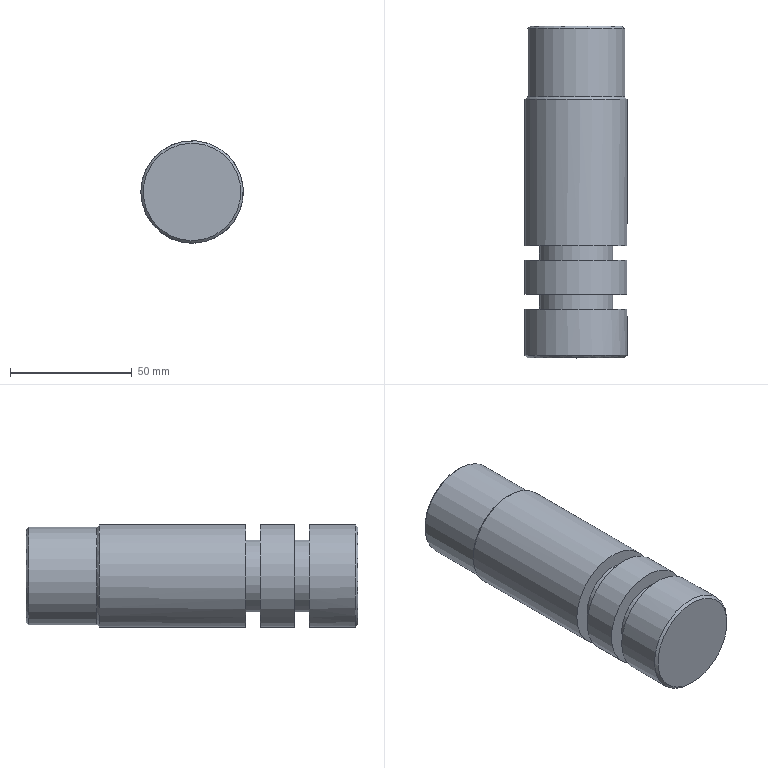Part | NX | features solid 2 | 1 solid | 15 faces | box 42 x 136 x 42 mm | volume 176350 mm3 | plane 6 | cylinder 6 | cone 3 | commonest cylinder face diameters 42 x3 30 x2 40 x1
STEP:
#1=CARTESIAN_POINT('',(-801.,-555.,180.));
#2=VERTEX_POINT('',#1);
#3=CARTESIAN_POINT('',(-780.,-555.,180.));
#4=DIRECTION('',(0.,1.,0.));
#5=DIRECTION('',(-1.,0.,0.));
#6=AXIS2_PLACEMENT_3D('',#3,#4,#5);
#7=CIRCLE('',#6,21.);
#8=EDGE_CURVE('',#2,#2,#7,.T.);
#9=ORIENTED_EDGE('',*,*,#8,.F.);
#10=EDGE_LOOP('',(#9));
#11=FACE_BOUND('',#10,.T.);
#12=CARTESIAN_POINT('',(-795.,-555.,180.));
#13=VERTEX_POINT('',#12);
#14=CARTESIAN_POINT('',(-780.,-555.,180.));
#15=DIRECTION('',(0.,1.,0.));
#16=DIRECTION('',(-1.,0.,0.));
#17=AXIS2_PLACEMENT_3D('',#14,#15,#16);
#18=CIRCLE('',#17,15.);
#19=EDGE_CURVE('',#13,#13,#18,.T.);
#20=ORIENTED_EDGE('',*,*,#19,.T.);
#21=EDGE_LOOP('',(#20));
#22=FACE_BOUND('',#21,.T.);
#23=CARTESIAN_POINT('',(-780.,-555.,180.));
#24=DIRECTION('',(0.,-1.,0.));
#25=DIRECTION('',(0.,0.,-1.));
#26=AXIS2_PLACEMENT_3D('',#23,#24,#25);
#27=PLANE('',#26);
#28=ADVANCED_FACE('',(#11,#22),#27,.T.);
#29=CARTESIAN_POINT('',(-801.,-535.,180.));
#30=VERTEX_POINT('',#29);
#31=CARTESIAN_POINT('',(-780.,-535.,180.));
#32=DIRECTION('',(0.,1.,0.));
#33=DIRECTION('',(-1.,0.,0.));
#34=AXIS2_PLACEMENT_3D('',#31,#32,#33);
#35=CIRCLE('',#34,21.);
#36=EDGE_CURVE('',#30,#30,#35,.T.);
#37=ORIENTED_EDGE('',*,*,#36,.F.);
#38=EDGE_LOOP('',(#37));
#39=FACE_BOUND('',#38,.T.);
#40=CARTESIAN_POINT('',(-795.,-535.,180.));
#41=VERTEX_POINT('',#40);
#42=CARTESIAN_POINT('',(-780.,-535.,180.));
#43=DIRECTION('',(0.,1.,0.));
#44=DIRECTION('',(-1.,0.,0.));
#45=AXIS2_PLACEMENT_3D('',#42,#43,#44);
#46=CIRCLE('',#45,15.);
#47=EDGE_CURVE('',#41,#41,#46,.T.);
#48=ORIENTED_EDGE('',*,*,#47,.T.);
#49=EDGE_LOOP('',(#48));
#50=FACE_BOUND('',#49,.T.);
#51=CARTESIAN_POINT('',(-780.,-535.,180.));
#52=DIRECTION('',(0.,-1.,0.));
#53=DIRECTION('',(0.,0.,-1.));
#54=AXIS2_PLACEMENT_3D('',#51,#52,#53);
#55=PLANE('',#54);
#56=ADVANCED_FACE('',(#39,#50),#55,.T.);
#57=CARTESIAN_POINT('',(-801.,-475.,180.));
#58=VERTEX_POINT('',#57);
#59=CARTESIAN_POINT('',(-780.,-475.,180.));
#60=DIRECTION('',(0.,1.,0.));
#61=DIRECTION('',(-1.,0.,0.));
#62=AXIS2_PLACEMENT_3D('',#59,#60,#61);
#63=CIRCLE('',#62,21.);
#64=EDGE_CURVE('',#58,#58,#63,.T.);
#65=ORIENTED_EDGE('',*,*,#64,.F.);
#66=EDGE_LOOP('',(#65));
#67=FACE_BOUND('',#66,.T.);
#68=ORIENTED_EDGE('',*,*,#36,.T.);
#69=EDGE_LOOP('',(#68));
#70=FACE_BOUND('',#69,.T.);
#71=CARTESIAN_POINT('',(-780.,-535.,180.));
#72=DIRECTION('',(0.,1.,0.));
#73=DIRECTION('',(0.,0.,1.));
#74=AXIS2_PLACEMENT_3D('',#71,#72,#73);
#75=CYLINDRICAL_SURFACE('',#74,21.);
#76=ADVANCED_FACE('',(#67,#70),#75,.T.);
#77=CARTESIAN_POINT('',(-795.,-541.,180.));
#78=VERTEX_POINT('',#77);
#79=CARTESIAN_POINT('',(-780.,-541.,180.));
#80=DIRECTION('',(0.,1.,0.));
#81=DIRECTION('',(-1.,0.,0.));
#82=AXIS2_PLACEMENT_3D('',#79,#80,#81);
#83=CIRCLE('',#82,15.);
#84=EDGE_CURVE('',#78,#78,#83,.T.);
#85=ORIENTED_EDGE('',*,*,#84,.T.);
#86=EDGE_LOOP('',(#85));
#87=FACE_BOUND('',#86,.T.);
#88=ORIENTED_EDGE('',*,*,#47,.F.);
#89=EDGE_LOOP('',(#88));
#90=FACE_BOUND('',#89,.T.);
#91=CARTESIAN_POINT('',(-780.,-541.,180.));
#92=DIRECTION('',(0.,1.,0.));
#93=DIRECTION('',(0.,0.,1.));
#94=AXIS2_PLACEMENT_3D('',#91,#92,#93);
#95=CYLINDRICAL_SURFACE('',#94,15.);
#96=ADVANCED_FACE('',(#87,#90),#95,.T.);
#97=CARTESIAN_POINT('',(-801.,-541.,180.));
#98=VERTEX_POINT('',#97);
#99=CARTESIAN_POINT('',(-780.,-541.,180.));
#100=DIRECTION('',(0.,1.,0.));
#101=DIRECTION('',(-1.,0.,0.));
#102=AXIS2_PLACEMENT_3D('',#99,#100,#101);
#103=CIRCLE('',#102,21.);
#104=EDGE_CURVE('',#98,#98,#103,.T.);
#105=ORIENTED_EDGE('',*,*,#104,.T.);
#106=EDGE_LOOP('',(#105));
#107=FACE_BOUND('',#106,.T.);
#108=ORIENTED_EDGE('',*,*,#84,.F.);
#109=EDGE_LOOP('',(#108));
#110=FACE_BOUND('',#109,.T.);
#111=CARTESIAN_POINT('',(-780.,-541.,180.));
#112=DIRECTION('',(0.,-1.,0.));
#113=DIRECTION('',(0.,0.,-1.));
#114=AXIS2_PLACEMENT_3D('',#111,#112,#113);
#115=PLANE('',#114);
#116=ADVANCED_FACE('',(#107,#110),#115,.F.);
#117=ORIENTED_EDGE('',*,*,#8,.T.);
#118=EDGE_LOOP('',(#117));
#119=FACE_BOUND('',#118,.T.);
#120=ORIENTED_EDGE('',*,*,#104,.F.);
#121=EDGE_LOOP('',(#120));
#122=FACE_BOUND('',#121,.T.);
#123=CARTESIAN_POINT('',(-780.,-555.,180.));
#124=DIRECTION('',(0.,1.,0.));
#125=DIRECTION('',(0.,0.,1.));
#126=AXIS2_PLACEMENT_3D('',#123,#124,#125);
#127=CYLINDRICAL_SURFACE('',#126,21.);
#128=ADVANCED_FACE('',(#119,#122),#127,.T.);
#129=CARTESIAN_POINT('',(-795.,-561.,180.));
#130=VERTEX_POINT('',#129);
#131=CARTESIAN_POINT('',(-780.,-561.,180.));
#132=DIRECTION('',(0.,1.,0.));
#133=DIRECTION('',(-1.,0.,0.));
#134=AXIS2_PLACEMENT_3D('',#131,#132,#133);
#135=CIRCLE('',#134,15.);
#136=EDGE_CURVE('',#130,#130,#135,.T.);
#137=ORIENTED_EDGE('',*,*,#136,.T.);
#138=EDGE_LOOP('',(#137));
#139=FACE_BOUND('',#138,.T.);
#140=ORIENTED_EDGE('',*,*,#19,.F.);
#141=EDGE_LOOP('',(#140));
#142=FACE_BOUND('',#141,.T.);
#143=CARTESIAN_POINT('',(-780.,-561.,180.));
#144=DIRECTION('',(0.,1.,0.));
#145=DIRECTION('',(0.,0.,1.));
#146=AXIS2_PLACEMENT_3D('',#143,#144,#145);
#147=CYLINDRICAL_SURFACE('',#146,15.);
#148=ADVANCED_FACE('',(#139,#142),#147,.T.);
#149=CARTESIAN_POINT('',(-801.,-561.,180.));
#150=VERTEX_POINT('',#149);
#151=CARTESIAN_POINT('',(-780.,-561.,180.));
#152=DIRECTION('',(0.,1.,0.));
#153=DIRECTION('',(-1.,0.,0.));
#154=AXIS2_PLACEMENT_3D('',#151,#152,#153);
#155=CIRCLE('',#154,21.);
#156=EDGE_CURVE('',#150,#150,#155,.T.);
#157=ORIENTED_EDGE('',*,*,#156,.T.);
#158=EDGE_LOOP('',(#157));
#159=FACE_BOUND('',#158,.T.);
#160=ORIENTED_EDGE('',*,*,#136,.F.);
#161=EDGE_LOOP('',(#160));
#162=FACE_BOUND('',#161,.T.);
#163=CARTESIAN_POINT('',(-780.,-561.,180.));
#164=DIRECTION('',(0.,-1.,0.));
#165=DIRECTION('',(0.,0.,-1.));
#166=AXIS2_PLACEMENT_3D('',#163,#164,#165);
#167=PLANE('',#166);
#168=ADVANCED_FACE('',(#159,#162),#167,.F.);
#169=CARTESIAN_POINT('',(-780.,-580.,159.));
#170=VERTEX_POINT('',#169);
#171=CARTESIAN_POINT('',(-780.,-580.,180.));
#172=DIRECTION('',(0.,1.,0.));
#173=DIRECTION('',(0.,0.,-1.));
#174=AXIS2_PLACEMENT_3D('',#171,#172,#173);
#175=CIRCLE('',#174,21.);
#176=EDGE_CURVE('',#170,#170,#175,.F.);
#177=ORIENTED_EDGE('',*,*,#176,.F.);
#178=EDGE_LOOP('',(#177));
#179=FACE_BOUND('',#178,.T.);
#180=ORIENTED_EDGE('',*,*,#156,.F.);
#181=EDGE_LOOP('',(#180));
#182=FACE_BOUND('',#181,.T.);
#183=CARTESIAN_POINT('',(-780.,-581.,180.));
#184=DIRECTION('',(0.,1.,0.));
#185=DIRECTION('',(0.,0.,1.));
#186=AXIS2_PLACEMENT_3D('',#183,#184,#185);
#187=CYLINDRICAL_SURFACE('',#186,21.);
#188=ADVANCED_FACE('',(#179,#182),#187,.T.);
#189=CARTESIAN_POINT('',(-780.,-581.,160.));
#190=VERTEX_POINT('',#189);
#191=CARTESIAN_POINT('',(-780.,-581.,180.));
#192=DIRECTION('',(0.,1.,0.));
#193=DIRECTION('',(0.,0.,-1.));
#194=AXIS2_PLACEMENT_3D('',#191,#192,#193);
#195=CIRCLE('',#194,20.);
#196=EDGE_CURVE('',#190,#190,#195,.T.);
#197=ORIENTED_EDGE('',*,*,#196,.F.);
#198=EDGE_LOOP('',(#197));
#199=FACE_BOUND('',#198,.T.);
#200=CARTESIAN_POINT('',(-780.,-581.,180.));
#201=DIRECTION('',(0.,-1.,0.));
#202=DIRECTION('',(0.,0.,-1.));
#203=AXIS2_PLACEMENT_3D('',#200,#201,#202);
#204=PLANE('',#203);
#205=ADVANCED_FACE('',(#199),#204,.T.);
#206=CARTESIAN_POINT('',(-780.,-474.,160.));
#207=VERTEX_POINT('',#206);
#208=CARTESIAN_POINT('',(-780.,-474.,180.));
#209=DIRECTION('',(0.,1.,0.));
#210=DIRECTION('',(0.,0.,-1.));
#211=AXIS2_PLACEMENT_3D('',#208,#209,#210);
#212=CIRCLE('',#211,20.);
#213=EDGE_CURVE('',#207,#207,#212,.F.);
#214=ORIENTED_EDGE('',*,*,#213,.F.);
#215=EDGE_LOOP('',(#214));
#216=FACE_BOUND('',#215,.T.);
#217=CARTESIAN_POINT('',(-780.,-446.,160.));
#218=VERTEX_POINT('',#217);
#219=CARTESIAN_POINT('',(-780.,-446.,180.));
#220=DIRECTION('',(0.,1.,0.));
#221=DIRECTION('',(0.,0.,-1.));
#222=AXIS2_PLACEMENT_3D('',#219,#220,#221);
#223=CIRCLE('',#222,20.);
#224=EDGE_CURVE('',#218,#218,#223,.T.);
#225=ORIENTED_EDGE('',*,*,#224,.F.);
#226=EDGE_LOOP('',(#225));
#227=FACE_BOUND('',#226,.T.);
#228=CARTESIAN_POINT('',(-780.,-405.,180.));
#229=DIRECTION('',(0.,-1.,0.));
#230=DIRECTION('',(0.,0.,-1.));
#231=AXIS2_PLACEMENT_3D('',#228,#229,#230);
#232=CYLINDRICAL_SURFACE('',#231,20.);
#233=ADVANCED_FACE('',(#216,#227),#232,.T.);
#234=CARTESIAN_POINT('',(-780.,-445.,161.));
#235=VERTEX_POINT('',#234);
#236=CARTESIAN_POINT('',(-780.,-445.,180.));
#237=DIRECTION('',(0.,1.,0.));
#238=DIRECTION('',(0.,0.,-1.));
#239=AXIS2_PLACEMENT_3D('',#236,#237,#238);
#240=CIRCLE('',#239,19.);
#241=EDGE_CURVE('',#235,#235,#240,.F.);
#242=ORIENTED_EDGE('',*,*,#241,.F.);
#243=EDGE_LOOP('',(#242));
#244=FACE_BOUND('',#243,.T.);
#245=CARTESIAN_POINT('',(-780.,-445.,180.));
#246=DIRECTION('',(0.,-1.,0.));
#247=DIRECTION('',(0.,0.,-1.));
#248=AXIS2_PLACEMENT_3D('',#245,#246,#247);
#249=PLANE('',#248);
#250=ADVANCED_FACE('',(#244),#249,.F.);
#251=ORIENTED_EDGE('',*,*,#241,.T.);
#252=EDGE_LOOP('',(#251));
#253=FACE_BOUND('',#252,.T.);
#254=ORIENTED_EDGE('',*,*,#224,.T.);
#255=EDGE_LOOP('',(#254));
#256=FACE_BOUND('',#255,.T.);
#257=CARTESIAN_POINT('',(-780.,-446.,180.));
#258=DIRECTION('',(0.,-1.,0.));
#259=DIRECTION('',(0.,0.,-1.));
#260=AXIS2_PLACEMENT_3D('',#257,#258,#259);
#261=CONICAL_SURFACE('',#260,20.,0.7854);
#262=ADVANCED_FACE('',(#253,#256),#261,.T.);
#263=ORIENTED_EDGE('',*,*,#213,.T.);
#264=EDGE_LOOP('',(#263));
#265=FACE_BOUND('',#264,.T.);
#266=ORIENTED_EDGE('',*,*,#64,.T.);
#267=EDGE_LOOP('',(#266));
#268=FACE_BOUND('',#267,.T.);
#269=CARTESIAN_POINT('',(-780.,-475.,180.));
#270=DIRECTION('',(0.,-1.,0.));
#271=DIRECTION('',(0.,0.,-1.));
#272=AXIS2_PLACEMENT_3D('',#269,#270,#271);
#273=CONICAL_SURFACE('',#272,21.,0.7854);
#274=ADVANCED_FACE('',(#265,#268),#273,.T.);
#275=ORIENTED_EDGE('',*,*,#176,.T.);
#276=EDGE_LOOP('',(#275));
#277=FACE_BOUND('',#276,.T.);
#278=ORIENTED_EDGE('',*,*,#196,.T.);
#279=EDGE_LOOP('',(#278));
#280=FACE_BOUND('',#279,.T.);
#281=CARTESIAN_POINT('',(-780.,-581.,180.));
#282=DIRECTION('',(0.,1.,0.));
#283=DIRECTION('',(0.,0.,1.));
#284=AXIS2_PLACEMENT_3D('',#281,#282,#283);
#285=CONICAL_SURFACE('',#284,20.,0.7854);
#286=ADVANCED_FACE('',(#277,#280),#285,.T.);
#287=CLOSED_SHELL('',(#28,#56,#76,#96,#116,#128,#148,#168,#188,#205,#233,#250,#262,#274,#286));
#288=MANIFOLD_SOLID_BREP('',#287);
#289=(LENGTH_UNIT()NAMED_UNIT(*)SI_UNIT(.MILLI.,.METRE.));
#290=UNCERTAINTY_MEASURE_WITH_UNIT(LENGTH_MEASURE(0.00001),#289,'','');
#291=(NAMED_UNIT(*)PLANE_ANGLE_UNIT()SI_UNIT($,.RADIAN.));
#292=(NAMED_UNIT(*)SI_UNIT($,.STERADIAN.)SOLID_ANGLE_UNIT());
#293=(GEOMETRIC_REPRESENTATION_CONTEXT(3)GLOBAL_UNCERTAINTY_ASSIGNED_CONTEXT((#290))GLOBAL_UNIT_ASSIGNED_CONTEXT((#289,#291,#292))REPRESENTATION_CONTEXT('',''));
#294=ADVANCED_BREP_SHAPE_REPRESENTATION('',(#288),#293);